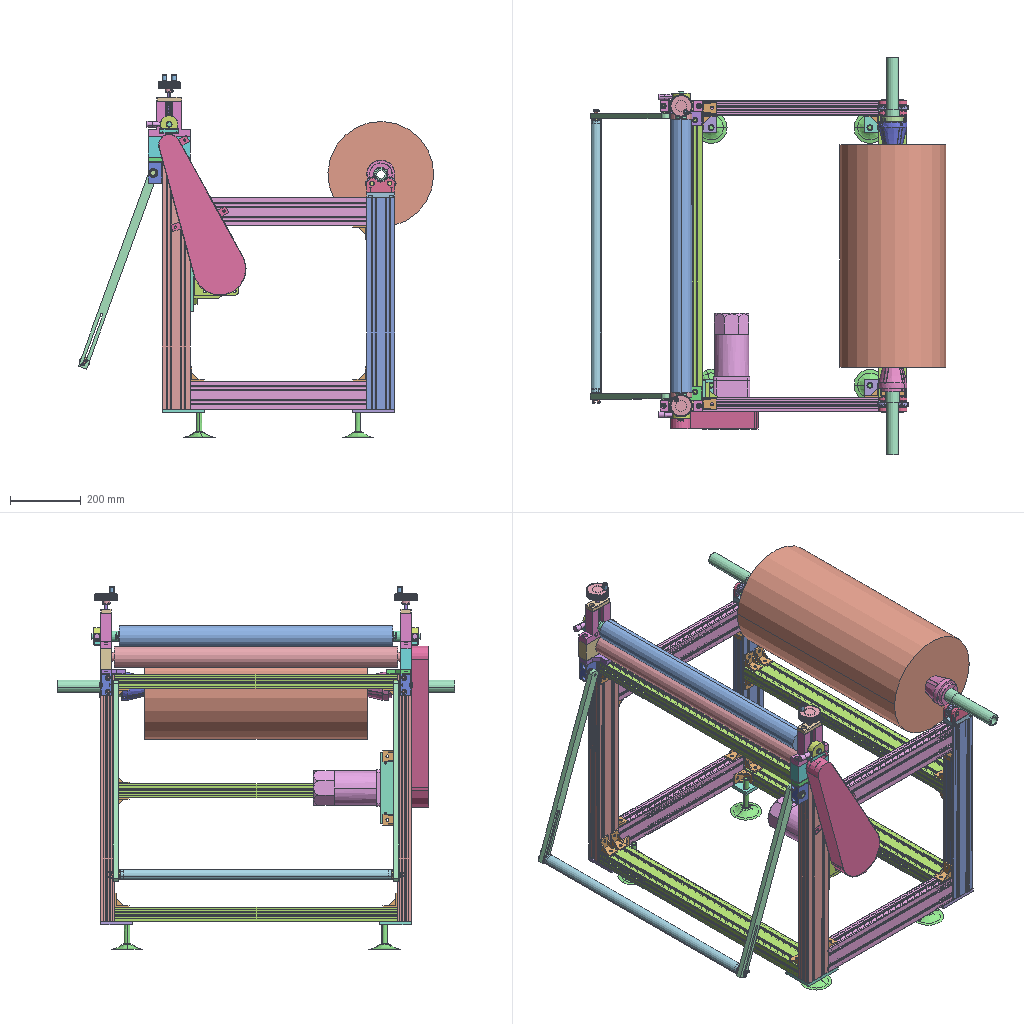Assembly | STEP file | 51 different items | 142 placed | box 1008 x 1128 x 1029 mm
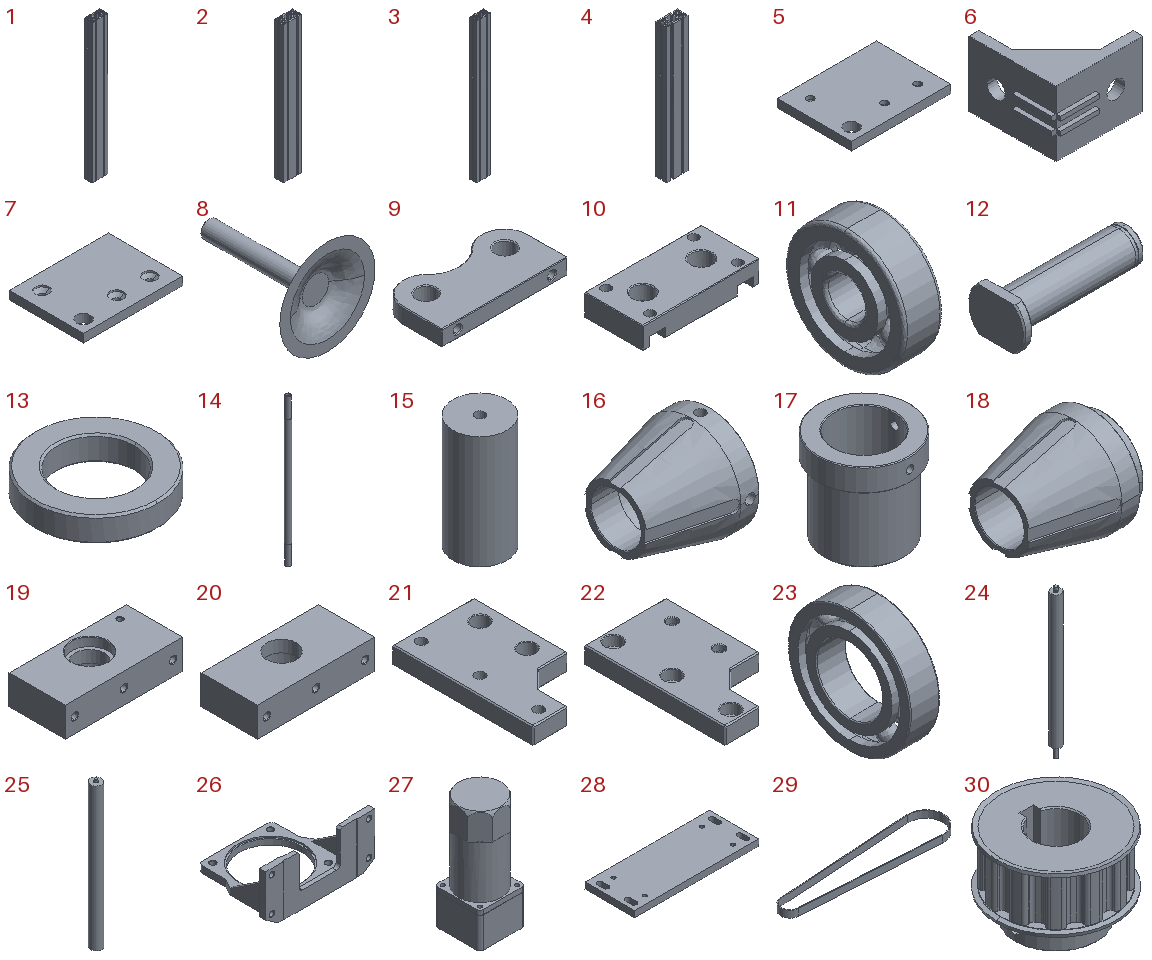Parts list (item | name | quantity | parent item | size | volume):
1 | 40x80 aluminium profile (L=700) | x2 | in Feed mechanism frame | 80 x 40 x 700 mm | 933883 mm3
2 | 40x80 aluminium profile (L=600) | x2 | in Feed mechanism frame | 80 x 40 x 600 mm | 800472 mm3
3 | 40x80 aluminium profile (L=800) | x4 | in Feed mechanism frame | 80 x 40 x 800 mm | 1067295 mm3
4 | 40x80 aluminium profile (L=500) | x4 | in Feed mechanism frame | 80 x 40 x 500 mm | 667060 mm3
5 | Foot cup plate | x2 | in Feed mechanism frame | 120 x 90 x 10 mm | 102433 mm3
6 | 40x40 angle bracket | x36 | in Feed mechanism frame, Feed mechanism | 42 x 42 x 30 mm | 11205 mm3
7 | Foot cup plate_MIR | x2 | in Feed mechanism frame | 120 x 90 x 10 mm | 102433 mm3
8 | M16 foot cup | x4 | in Feed mechanism frame | 90 x 113.5 x 90 mm | 31206 mm3
9 | Roll shaft support seat | x4 | in Roll shaft support assembly | 80 x 40 x 10 mm | 25332 mm3
10 | Roll shaft support base plate | x2 | in Roll shaft support assembly | 80 x 40 x 15 mm | 40545 mm3
11 | Rolling bearing GB_T 276-94 6301 | x4 | in Roll shaft support assembly | - | -
12 | Roll shaft support bearing shaft | x4 | in Roll shaft support assembly | 46 x 20 x 15 mm | 5646 mm3
13 | Bearing locating ring | x8 | in Roll shaft support assembly | 20 x 20 x 4 mm | 756.574 mm3
14 | Roll shaft | x1 | in Feed mechanism | 40 x 40 x 1128 mm | 818698 mm3
15 | Coil stock | x1 | in Feed mechanism | 300 x 300 x 630 mm | 43035303 mm3
16 | Coil positioning piece 1 | x1 | in Feed mechanism | 75 x 80 x 80 mm | 140418 mm3
17 | Coil positioning adjuster | x1 | in Feed mechanism | 60 x 60 x 60 mm | 62041 mm3
18 | Coil positioning piece 2 | x1 | in Feed mechanism | 85 x 80 x 80 mm | 199257 mm3
19 | Roller base | x1 | in Feed mechanism | 120 x 57 x 30 mm | 174440 mm3
20 | Roller base 2 | x1 | in Feed mechanism | 120 x 57 x 30 mm | 174618 mm3
21 | Roller base fixing plate | x1 | in Feed mechanism | 70 x 120 x 15 mm | 94561 mm3
22 | Roller base fixing plate_MIR | x1 | in Feed mechanism | 70 x 120 x 15 mm | 94561 mm3
23 | Rolling bearing GB_T 276-94 61904 | x4 | in Feed mechanism | - | -
24 | Main roller | x1 | in Feed mechanism | 60 x 60 x 898 mm | 2307157 mm3
25 | Auxiliary roller 3 | x1 | in Feed mechanism | 60 x 60 x 799 mm | 2193510 mm3
26 | DDK motor base (RAL100) | x1 | in Feed mechanism | 160 x 125.5 x 75 mm | 142443 mm3
27 | DDK250W50 electromagnetic brake motor | x1 | in Feed mechanism | 104 x 104 x 302.5 mm | 2241190 mm3
28 | Feed motor plate | x1 | in Feed mechanism | 200 x 80 x 10 mm | 153554 mm3
29 | Timing belt_3 | x1 | in Timing belt conveyor_3 | 455.684 x 99.713 x 19.05 mm | 38426 mm3
30 | Timing pulley 1_3 | x1 | in Timing belt conveyor_3 | 51.203 x 51.203 x 35.319 mm | 36393 mm3
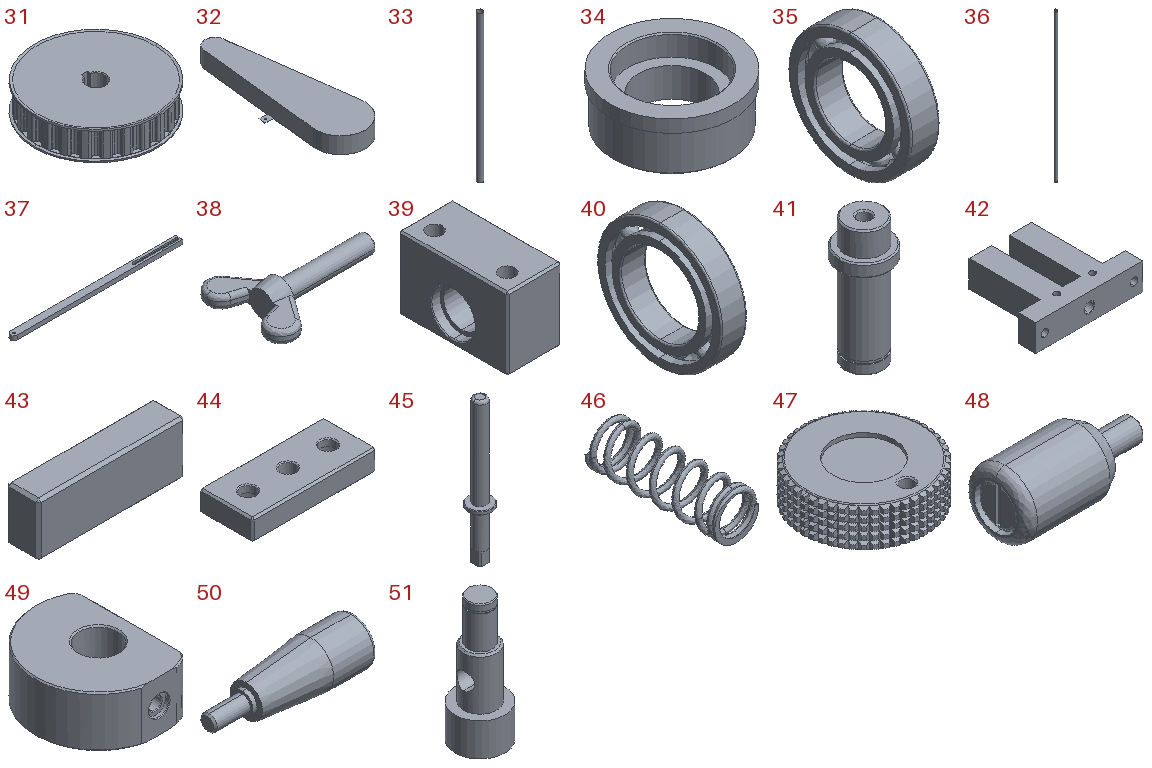31 | Timing pulley 2_3 | x1 | in Timing belt conveyor_3 | 99.713 x 99.713 x 35.319 mm | 162767 mm3
32 | Protective cover | x1 | in Feed mechanism | 167.34 x 485.19 x 50 mm | 105387 mm3
33 | Guide roller housing 3 | x1 | in 25 | 29.5 x 29.5 x 770 mm | 45363 mm3
34 | Guide roller bearing seat | x2 | in 25 | 29.5 x 29.5 x 12 mm | 4526 mm3
35 | Rolling bearing GB_T 276-94 61801 | x2 | in 25 | - | -
36 | Guide roller shaft 4 | x1 | in 25 | 12 x 12 x 790 mm | 88894 mm3
37 | Feed swing arm | x2 | in 25 | 600 x 25 x 15 mm | 204711 mm3
38 | JIS B 1184 - M5 x 25 | x2 | in 25 | 37 x 25 x 8.5 mm | 1182 mm3
39 | Feed swing arm fixing piece | x2 | in 25 | 30 x 60 x 40 mm | 54813 mm3
40 | Rolling bearing GB_T 276-94 61802 | x8 | in 25, Feed mechanism | - | -
41 | Swing arm pivot shaft | x2 | in 25 | 20 x 20 x 49.5 mm | 9151 mm3
42 | Pressure plate fixing seat | x2 | in Pressure roller mechanism | 120 x 100 x 30 mm | 182269 mm3
43 | Cam top plate | x2 | in Pressure roller mechanism | 55 x 12 x 20 mm | 12439 mm3
44 | Adjusting plate | x2 | in Pressure roller mechanism | 70 x 30 x 12 mm | 21378 mm3
45 | Adjusting screw | x2 | in Pressure roller mechanism | 18 x 18 x 110 mm | 8965 mm3
46 | Compression spring 1_1 | x2 | in Compression spring_1 | - | 1226 mm3
47 | CHBK631_1 | x2 | in CHBK63_1 | 63 x 63 x 29 mm | 58245 mm3
48 | CHBK632_1 | x2 | in CHBK63_1 | 29.8 x 14 x 14 mm | 3166 mm3
49 | Pressure roller | x2 | in Feed mechanism | 38 x 49 x 20 mm | 27809 mm3
50 | GRAM6 | x2 | in Feed mechanism | 54.5 x 17 x 17 mm | 8003 mm3
51 | Shaft end fixing piece | x2 | in Feed mechanism | 30 x 30 x 76 mm | 20757 mm3
Placements (level | parent | child | x y z in mm | rotation matrix by rows):
1 | Feed mechanism | Feed mechanism frame | -0.0 -0.0 -0.0 | 1 0 0 0 1 0 0 0 1
2 | Feed mechanism frame | 40x80 aluminium profile (L=700) | -26.052 -22.306 -747.237 | 1 0 0 0 1 0 0 0 1
2 | Feed mechanism frame | 40x80 aluminium profile (L=700) | -26.052 817.694 -747.237 | 1 0 0 0 1 0 0 0 1
2 | Feed mechanism frame | 40x80 aluminium profile (L=600) | 553.948 -22.306 -747.237 | 1 0 0 0 1 0 0 0 1
2 | Feed mechanism frame | 40x80 aluminium profile (L=600) | 553.948 817.694 -747.237 | 1 0 0 0 1 0 0 0 1
2 | Feed mechanism frame | 40x80 aluminium profile (L=800) | -26.052 17.694 -707.237 | 1 0 0 0 0 1 0 -1 -0
2 | Feed mechanism frame | 40x80 aluminium profile (L=800) | 553.948 17.694 -707.237 | 1 0 0 0 0 1 0 -1 -0
2 | Feed mechanism frame | 40x80 aluminium profile (L=800) | -26.052 17.694 -47.237 | 1 0 0 0 0 1 0 -1 -0
2 | Feed mechanism frame | 40x80 aluminium profile (L=500) | 553.948 817.694 -227.237 | 0 0 -1 0 1 0 1 0 0
2 | Feed mechanism frame | 40x80 aluminium profile (L=500) | 553.948 -22.306 -227.237 | 0 0 -1 0 1 0 1 0 0
2 | Feed mechanism frame | 40x80 aluminium profile (L=500) | 553.948 -22.306 -747.237 | 0 0 -1 0 1 0 1 0 0
2 | Feed mechanism frame | 40x80 aluminium profile (L=500) | 553.948 817.694 -747.237 | 0 0 -1 0 1 0 1 0 0
2 | Feed mechanism frame | Foot cup plate | 93.948 67.694 -757.237 | -1 0 0 0 -1 0 0 0 1
2 | Feed mechanism frame | Foot cup plate | 513.948 767.694 -757.237 | 1 0 0 0 1 0 0 0 1
2 | Feed mechanism frame | 40x40 angle bracket | 53.948 12.694 -107.237 | 1 0 0 0 0 -1 0 1 0
2 | Feed mechanism frame | 40x40 angle bracket | 53.948 852.694 -107.237 | 1 0 0 0 0 -1 0 1 0
2 | Feed mechanism frame | 40x40 angle bracket | 93.948 852.694 -227.237 | 0 1 0 0 0 -1 -1 0 -0
2 | Feed mechanism frame | 40x40 angle bracket | 93.948 12.694 -227.237 | 0 1 0 0 0 -1 -1 0 0
2 | Feed mechanism frame | 40x40 angle bracket | 93.948 822.694 -667.237 | 0 1 0 0 0 1 1 0 -0
2 | Feed mechanism frame | 40x40 angle bracket | -21.052 777.694 -707.237 | 0 0 1 0 -1 0 1 0 -0
2 | Feed mechanism frame | 40x40 angle bracket | 18.948 777.694 -707.237 | 0 0 1 0 -1 0 1 0 -0
2 | Feed mechanism frame | 40x40 angle bracket | -21.052 17.694 -667.237 | 0 0 1 1 0 0 0 1 -0
2 | Feed mechanism frame | 40x40 angle bracket | 18.948 17.694 -667.237 | 0 0 1 1 0 0 0 1 0
2 | Feed mechanism frame | 40x40 angle bracket | 53.948 777.694 -712.237 | 1 0 0 0 -1 0 0 0 -1
2 | Feed mechanism frame | 40x40 angle bracket | 93.948 17.694 -712.237 | 0 1 0 1 0 0 0 0 -1
2 | Feed mechanism frame | 40x40 angle bracket | 53.948 12.694 -627.237 | 1 0 0 0 0 -1 0 1 0
2 | Feed mechanism frame | 40x40 angle bracket | 8.948 777.694 -87.237 | 0 0 -1 0 -1 0 -1 0 -0
2 | Feed mechanism frame | 40x40 angle bracket | 48.948 777.694 -87.237 | 0 0 -1 0 -1 0 -1 0 0
2 | Feed mechanism frame | 40x40 angle bracket | -21.052 57.694 -87.237 | 0 0 1 0 1 0 -1 0 -0
2 | Feed mechanism frame | 40x40 angle bracket | 18.948 57.694 -87.237 | 0 0 1 0 1 0 -1 0 -0
2 | Feed mechanism frame | 40x40 angle bracket | 513.948 12.694 -667.237 | 0 -1 0 0 0 -1 1 0 -0
2 | Feed mechanism frame | 40x40 angle bracket | 513.948 17.694 -742.237 | 0 -1 0 1 0 0 0 0 1
2 | Feed mechanism frame | 40x40 angle bracket | 588.948 57.694 -707.237 | 0 0 -1 0 1 0 1 0 0
2 | Feed mechanism frame | 40x40 angle bracket | 628.948 57.694 -707.237 | 0 0 -1 0 1 0 1 0 0
2 | Feed mechanism frame | 40x40 angle bracket | 553.948 822.694 -627.237 | -1 0 0 0 0 1 0 1 -0
2 | Feed mechanism frame | 40x40 angle bracket | 513.948 817.694 -712.237 | 0 -1 0 -1 0 0 0 0 -1
2 | Feed mechanism frame | 40x40 angle bracket | 558.948 777.694 -707.237 | 0 0 1 0 -1 0 1 0 -0
2 | Feed mechanism frame | 40x40 angle bracket | 598.948 777.694 -707.237 | 0 0 1 0 -1 0 1 0 -0
2 | Feed mechanism frame | 40x40 angle bracket | 553.948 852.694 -267.237 | -1 0 0 0 0 -1 0 -1 0
2 | Feed mechanism frame | 40x40 angle bracket | 553.948 12.694 -267.237 | -1 0 0 0 0 -1 0 -1 -0
2 | Feed mechanism frame | 40x80 aluminium profile (L=800) | 553.948 17.694 -357.237 | 1 0 0 0 0 1 0 -1 -0
2 | Feed mechanism frame | 40x40 angle bracket | 598.948 777.694 -357.237 | 0 0 1 0 -1 0 1 0 -0
2 | Feed mechanism frame | 40x40 angle bracket | 558.948 777.694 -357.237 | 0 0 1 0 -1 0 1 0 -0
2 | Feed mechanism frame | 40x40 angle bracket | 588.948 777.694 -397.237 | 0 0 -1 0 -1 0 -1 0 0
2 | Feed mechanism frame | 40x40 angle bracket | 628.948 777.694 -397.237 | 0 0 -1 0 -1 0 -1 0 0
2 | Feed mechanism frame | 40x40 angle bracket | 558.948 17.694 -317.237 | 0 0 1 1 0 0 0 1 -0
2 | Feed mechanism frame | 40x40 angle bracket | 598.948 17.694 -317.237 | 0 0 1 1 0 0 0 1 -0
2 | Feed mechanism frame | 40x40 angle bracket | 628.948 17.694 -437.237 | 0 0 -1 1 0 0 0 -1 0
2 | Feed mechanism frame | 40x40 angle bracket | 558.948 57.694 -397.237 | 0 0 1 0 1 0 -1 0 -0
2 | Feed mechanism frame | Foot cup plate_MIR | 93.948 767.694 -757.237 | -1 0 0 0 1 0 0 0 -1
2 | Feed mechanism frame | Foot cup plate_MIR | 513.948 67.694 -757.237 | 1 0 0 0 -1 0 0 0 -1
2 | Feed mechanism frame | M16 foot cup | 28.846 219.519 -924.74 | -0.2876 0 0.9577 0.9577 0 0.2876 0 1 0
2 | Feed mechanism frame | M16 foot cup | 703.134 52.694 -924.74 | 1 0 0 0 0 -1 0 1 0
2 | Feed mechanism frame | M16 foot cup | 253.134 782.694 -924.74 | 1 0 0 0 0 -1 0 1 0
2 | Feed mechanism frame | M16 foot cup | 703.134 782.694 -924.74 | 1 0 0 0 0 -1 0 1 0
1 | Feed mechanism | Roll shaft support assembly | 605.113 847.694 -152.986 | -1 0 0 0 0 1 0 1 -0
2 | Roll shaft support assembly | Roll shaft support seat | -28.835 20.749 0.0 | 1 0 0 0 1 0 0 0 1
2 | Roll shaft support assembly | Roll shaft support base plate | -28.835 5.749 10.0 | 1 0 0 0 0 1 0 -1 -0
2 | Roll shaft support assembly | Roll shaft support seat | -28.835 20.749 -30.0 | 1 0 0 0 1 0 0 0 1
2 | Roll shaft support assembly | Rolling bearing GB_T 276-94 6301 | 36.165 45.749 -4.0 | 0 0 1 0 1 0 -1 0 -0
2 | Roll shaft support assembly | Rolling bearing GB_T 276-94 6301 | -13.835 45.749 -4.0 | 0 0 1 0 1 0 -1 0 -0
2 | Roll shaft support assembly | Roll shaft support bearing shaft | 36.165 45.749 -33.0 | 0 0 -1 0 1 0 1 0 0
2 | Roll shaft support assembly | Roll shaft support bearing shaft | -13.835 45.749 -33.0 | 0 0 -1 0 1 0 1 0 0
2 | Roll shaft support assembly | Bearing locating ring | 36.165 45.749 -16.0 | 1 0 0 0 -1 0 0 0 -1
2 | Roll shaft support assembly | Bearing locating ring | 36.165 45.749 0.0 | 1 0 0 0 -1 0 0 0 -1
2 | Roll shaft support assembly | Bearing locating ring | -13.835 45.749 -20.0 | 1 0 0 0 1 0 0 0 1
2 | Roll shaft support assembly | Bearing locating ring | -13.835 45.749 -0.0 | 1 0 0 0 -1 0 0 0 -1
1 | Feed mechanism | Roll shaft support assembly | 582.783 -12.306 -152.986 | 1 0 0 0 0 -1 0 1 0
2 | Roll shaft support assembly | Roll shaft support seat | -28.835 20.749 0.0 | 1 0 0 0 1 0 0 0 1
2 | Roll shaft support assembly | Roll shaft support base plate | -28.835 5.749 10.0 | 1 0 0 0 0 1 0 -1 -0
2 | Roll shaft support assembly | Roll shaft support seat | -28.835 20.749 -30.0 | 1 0 0 0 1 0 0 0 1
2 | Roll shaft support assembly | Rolling bearing GB_T 276-94 6301 | 36.165 45.749 -4.0 | 0 0 1 0 1 0 -1 0 -0
2 | Roll shaft support assembly | Rolling bearing GB_T 276-94 6301 | -13.835 45.749 -4.0 | 0 0 1 0 1 0 -1 0 -0
2 | Roll shaft support assembly | Roll shaft support bearing shaft | 36.165 45.749 -33.0 | 0 0 -1 0 1 0 1 0 0
2 | Roll shaft support assembly | Roll shaft support bearing shaft | -13.835 45.749 -33.0 | 0 0 -1 0 1 0 1 0 0
2 | Roll shaft support assembly | Bearing locating ring | 36.165 45.749 -16.0 | 1 0 0 0 -1 0 0 0 -1
2 | Roll shaft support assembly | Bearing locating ring | 36.165 45.749 0.0 | 1 0 0 0 -1 0 0 0 -1
2 | Roll shaft support assembly | Bearing locating ring | -13.835 45.749 -20.0 | 1 0 0 0 1 0 0 0 1
2 | Roll shaft support assembly | Bearing locating ring | -13.835 45.749 -0.0 | 1 0 0 0 -1 0 0 0 -1
1 | Feed mechanism | Roll shaft | 593.948 831.694 -81.333 | 0.9883 -0.1522 0 0 0 -1 0.1522 0.9883 0
1 | Feed mechanism | Coil stock | 593.948 102.694 -81.333 | 0.9992 -0.03997 0 0 0 1 -0.03997 -0.9992 -0
1 | Feed mechanism | Coil positioning piece 1 | 593.948 722.843 -81.333 | 0 -0.7984 0.6022 1 0 0 0 0.6022 0.7984
1 | Feed mechanism | Coil positioning adjuster | 593.948 752.843 -81.333 | -0.7259 0.6878 0 0 0 1 0.6878 0.7259 0
1 | Feed mechanism | Coil positioning piece 2 | 593.948 117.695 -81.333 | 0 0.8112 -0.5848 -1 0 0 0 0.5848 0.8112
1 | Feed mechanism | Roller base | -66.052 -7.306 -32.237 | 1 0 0 0 0 -1 0 1 0
1 | Feed mechanism | Roller base 2 | 53.948 842.694 -32.237 | -1 0 0 0 0 1 0 1 -0
1 | Feed mechanism | Roller base fixing plate | -66.052 857.694 -47.237 | 0 1 0 -1 0 0 0 0 1
1 | Feed mechanism | Roller base fixing plate_MIR | -66.052 -22.306 -47.237 | 0 1 0 1 0 0 0 0 -1
1 | Feed mechanism | Rolling bearing GB_T 276-94 61904 | -6.052 7.694 2.763 | 0 0.9854 0.1703 -1 0 0 0 -0.1703 0.9854
1 | Feed mechanism | Rolling bearing GB_T 276-94 61904 | -6.052 827.694 2.763 | 0 -0.7592 0.6509 1 0 0 0 0.6509 0.7592
1 | Feed mechanism | Main roller | -6.052 15.194 2.763 | -0.3761 0.9266 0 0 0 1 0.9266 0.3761 -0
1 | Feed mechanism | Rolling bearing GB_T 276-94 61904 | -6.052 845.694 2.763 | 0 -0.9115 -0.4113 -1 0 0 0 0.4113 -0.9115
1 | Feed mechanism | Rolling bearing GB_T 276-94 61904 | -6.052 -13.306 2.763 | 0 -0.9115 0.4113 -1 0 0 0 -0.4113 -0.9115
1 | Feed mechanism | Auxiliary roller 3 | -6.052 30.694 60.263 | 0 -1 0 0 0 1 -1 0 -0
1 | Feed mechanism | DDK motor base (RAL100) | 64.948 -15.306 -423.548 | 0 1 0 0 0 1 1 0 -0
1 | Feed mechanism | DDK250W50 electromagnetic brake motor | 136.948 -5.306 -369.548 | -1 0 0 0 0 1 0 1 0
1 | Feed mechanism | Feed motor plate | 53.948 64.694 -469.548 | 0 0 1 0 -1 0 1 0 -0
1 | Feed mechanism | Timing belt conveyor_3 | -67.475 100.469 -17.719 | 0.3901 0 -0.9208 0 1 0 0.9208 0 0.3901
2 | Timing belt conveyor_3 | Timing belt_3 | -27.822 -141.345 -119.343 | -0.7064 0.7078 0 0 0 -1 -0.7078 -0.7064 -0
2 | Timing belt conveyor_3 | Timing pulley 1_3 | 42.822 -141.345 -48.566 | -0.7064 0.7078 0 0 0 -1 -0.7078 -0.7064 -0
2 | Timing belt conveyor_3 | Timing pulley 2_3 | -225.786 -141.345 -317.679 | -0.7064 0.7078 0 0 0 -1 -0.7078 -0.7064 -0
1 | Feed mechanism | Protective cover | -6.052 -22.306 2.763 | 0.9317 -0.3632 0 0 0 -1 0.3632 0.9317 -0
1 | Feed mechanism | Auxiliary roller 3 | -26.052 857.694 -47.237 | -1 0 0 0 0 -1 0 -1 0
2 | Auxiliary roller 3 | Guide roller housing 3 | 220.9 567.94 55.0 | -0.9333 0.3591 0 -0.3591 -0.9333 0 0 0 1
2 | Auxiliary roller 3 | Guide roller bearing seat | 220.9 567.94 816.0 | -0.4356 0.9001 0 -0.9001 -0.4356 0 0 0 1
2 | Auxiliary roller 3 | Guide roller bearing seat | 220.9 567.94 64.0 | 0.712 -0.7022 0 -0.7022 -0.712 0 0 0 -1
2 | Auxiliary roller 3 | Rolling bearing GB_T 276-94 61801 | 220.9 567.94 52.0 | 0 0.9695 0.2452 0 -0.2452 0.9695 1 0 0
2 | Auxiliary roller 3 | Rolling bearing GB_T 276-94 61801 | 220.9 567.94 828.0 | 0 0.9966 -0.08277 0 -0.08277 -0.9966 -1 0 -0
2 | Auxiliary roller 3 | Guide roller shaft 4 | 220.9 567.94 45.0 | -0.9397 -0.342 0 0.342 -0.9397 0 0 0 1
2 | Auxiliary roller 3 | Feed swing arm | 8.979 22.529 845.0 | 0.342 0.9397 0 0.9397 -0.342 0 0 0 -1
2 | Auxiliary roller 3 | Feed swing arm | 32.471 13.979 35.0 | 0.342 -0.9397 0 0.9397 0.342 0 0 0 1
2 | Auxiliary roller 3 | JIS B 1184 - M5 x 25 | 220.9 567.94 845.0 | 0 -0.8388 -0.5444 0 -0.5444 0.8388 -1 0 -0
2 | Auxiliary roller 3 | JIS B 1184 - M5 x 25 | 220.9 567.94 35.0 | 0 -0.5654 0.8248 0 -0.8248 -0.5654 1 0 0
2 | Auxiliary roller 3 | Feed swing arm fixing piece | 40.0 0.0 850.0 | 0 0 -1 0 1 0 1 0 0
2 | Auxiliary roller 3 | Feed swing arm fixing piece | 40.0 60.0 30.0 | 0 0 -1 0 -1 0 -1 0 0
2 | Auxiliary roller 3 | Rolling bearing GB_T 276-94 61802 | 25.0 30.0 855.0 | 0 -0.9688 -0.2477 0 -0.2477 0.9688 -1 0 -0
2 | Auxiliary roller 3 | Rolling bearing GB_T 276-94 61802 | 25.0 30.0 25.0 | 0 -0.9985 0.05385 0 -0.05385 -0.9985 1 0 -0
2 | Auxiliary roller 3 | Rolling bearing GB_T 276-94 61802 | 25.0 30.0 880.0 | 0 -0.9688 -0.2477 0 -0.2477 0.9688 -1 0 -0
2 | Auxiliary roller 3 | Rolling bearing GB_T 276-94 61802 | 25.0 30.0 0.0 | 0 -0.9985 0.05385 0 -0.05385 -0.9985 1 0 0
2 | Auxiliary roller 3 | Swing arm pivot shaft | 25.0 30.0 885.0 | 0.6219 0.7831 0 0.7831 -0.6219 0 0 0 -1
2 | Auxiliary roller 3 | Swing arm pivot shaft | 25.0 30.0 -5.0 | -0.05385 -0.9985 0 0.9985 -0.05385 0 0 0 1
1 | Feed mechanism | 40x40 angle bracket | 13.948 17.694 -294.548 | 0 -1 0 1 0 0 0 0 1
1 | Feed mechanism | 40x40 angle bracket | 13.948 17.694 -474.548 | 0 -1 0 1 0 0 0 0 1
1 | Feed mechanism | Pressure roller mechanism | -41.052 7.694 24.763 | 1 0 0 0 0 -1 0 1 0
2 | Pressure roller mechanism | Pressure plate fixing seat | -0.0 -0.0 -0.0 | 1 0 0 0 1 0 0 0 1
2 | Pressure roller mechanism | Cam top plate | 7.5 10.5 30.0 | 1 0 0 0 1 0 0 0 1
2 | Pressure roller mechanism | Adjusting plate | 0.0 112.0 0.0 | 1 0 0 0 0 -1 0 1 0
2 | Pressure roller mechanism | Adjusting screw | 35.0 100.0 15.0 | 0.4116 -0.9114 0 0 0 -1 0.9114 0.4116 0
2 | Pressure roller mechanism | Compression spring_1 | 35.0 90.258 15.0 | 1 0 0 0 -1 0 0 0 -1
3 | Compression spring_1 | Compression spring 1_1 | 0.0 -0.0 -0.0 | 1 0 0 0 1 0 0 0 1
2 | Pressure roller mechanism | CHBK63_1 | 35.0 146.0 15.0 | -0.7973 0.6035 0 0 0 1 0.6035 0.7973 -0
3 | CHBK63_1 | CHBK631_1 | -0.0 -0.0 -0.0 | 1 0 0 0 1 0 0 0 1
3 | CHBK63_1 | CHBK632_1 | 0.0 -22.0 30.8 | 0 0 -1 0 -1 0 -1 0 -0
1 | Feed mechanism | Pressure roller mechanism | 28.948 827.694 24.763 | -1 0 0 0 0 1 0 1 -0
2 | Pressure roller mechanism | Pressure plate fixing seat | -0.0 -0.0 -0.0 | 1 0 0 0 1 0 0 0 1
2 | Pressure roller mechanism | Cam top plate | 7.5 10.5 30.0 | 1 0 0 0 1 0 0 0 1
2 | Pressure roller mechanism | Adjusting plate | 0.0 112.0 0.0 | 1 0 0 0 0 -1 0 1 0
2 | Pressure roller mechanism | Adjusting screw | 35.0 100.0 15.0 | 0.4116 -0.9114 0 0 0 -1 0.9114 0.4116 0
2 | Pressure roller mechanism | Compression spring_1 | 35.0 90.258 15.0 | 1 0 0 0 -1 0 0 0 -1
3 | Compression spring_1 | Compression spring 1_1 | 0.0 -0.0 -0.0 | 1 0 0 0 1 0 0 0 1
2 | Pressure roller mechanism | CHBK63_1 | 35.0 146.0 15.0 | -0.7973 0.6035 0 0 0 1 0.6035 0.7973 -0
3 | CHBK63_1 | CHBK631_1 | -0.0 -0.0 -0.0 | 1 0 0 0 1 0 0 0 1
3 | CHBK63_1 | CHBK632_1 | 0.0 -22.0 30.8 | 0 0 -1 0 -1 0 -1 0 -0
1 | Feed mechanism | Pressure roller | -6.052 -22.806 60.263 | 0 1 0 0 0 -1 -1 0 0
1 | Feed mechanism | Pressure roller | -6.052 878.194 60.263 | 0 1 0 0 0 -1 -1 0 0
1 | Feed mechanism | GRAM6 | -30.052 868.194 60.263 | -1 0 0 0 1 0 0 0 -1
1 | Feed mechanism | GRAM6 | -30.052 -32.806 60.263 | -1 0 0 0 0.2985 -0.9544 0 -0.9544 -0.2985
1 | Feed mechanism | Shaft end fixing piece | -6.052 807.194 60.263 | 0 1 0 0 0 1 1 0 -0
1 | Feed mechanism | Shaft end fixing piece | -6.052 28.194 60.263 | 0 1 0 0 0 -1 -1 0 0
1 | Feed mechanism | Rolling bearing GB_T 276-94 61802 | -6.052 812.194 60.263 | 0 -1 0 1 0 0 0 0 1
1 | Feed mechanism | Rolling bearing GB_T 276-94 61802 | -6.052 807.194 60.263 | 0 -1 0 1 0 0 0 0 1
1 | Feed mechanism | Rolling bearing GB_T 276-94 61802 | -6.052 23.194 60.263 | 0 1 0 -1 0 0 0 0 1
1 | Feed mechanism | Rolling bearing GB_T 276-94 61802 | -6.052 28.194 60.263 | 0 1 0 -1 0 0 0 0 1